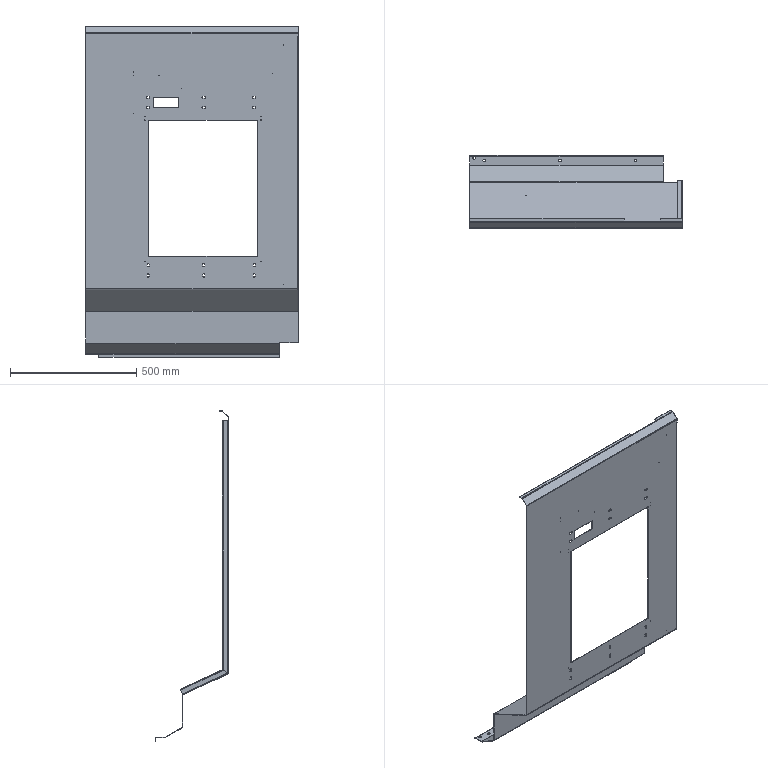Part | NX | features solid 2 | 1 solid | 180 faces | box 843 x 290 x 1310 mm | volume 2157482 mm3 | cylinder 90 | plane 86 | spline 4 | commonest cylinder face diameters 1 x30 7 x30 4 x11 8 x11 10 x8